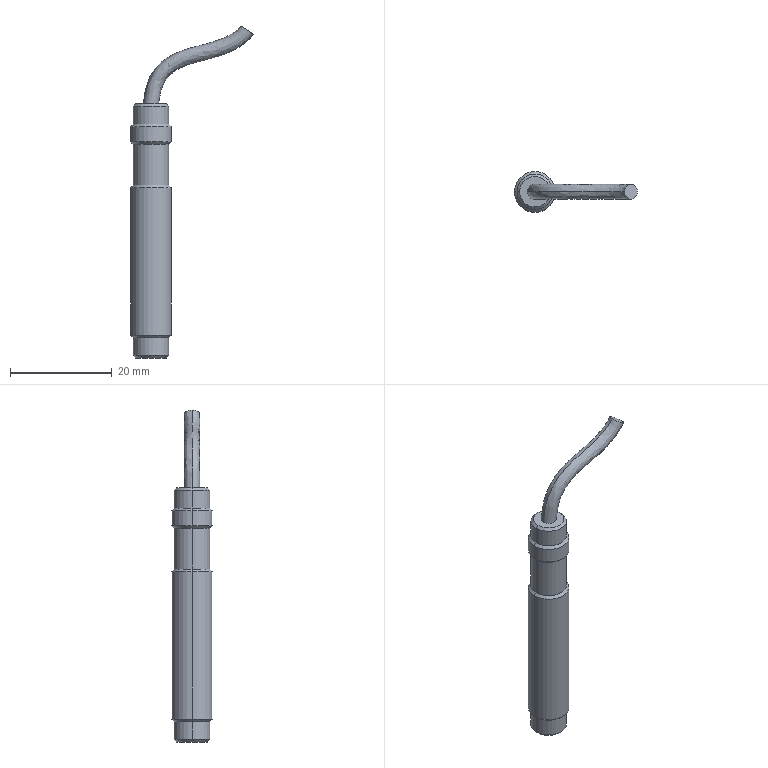Part | STEP file | 11-PSC0802-N.11 | 1 solid | 27 faces | box 24.159 x 8 x 65.269 mm | volume 2489 mm3 | cone 12 | cylinder 10 | plane 3 | spline 2 | commonest cylinder face diameters 7 x6 8 x4
STEP:
#1=CARTESIAN_POINT('',(3.5,0.,4.));
#2=VERTEX_POINT('',#1);
#3=CARTESIAN_POINT('',(-3.5,0.,4.));
#4=VERTEX_POINT('',#3);
#5=CARTESIAN_POINT('',(0.,0.,4.));
#6=DIRECTION('',(0.,0.,1.));
#7=DIRECTION('',(1.,0.,0.));
#8=AXIS2_PLACEMENT_3D('',#5,#6,#7);
#9=CIRCLE('',#8,3.5);
#10=EDGE_CURVE('',#2,#4,#9,.T.);
#11=ORIENTED_EDGE('',*,*,#10,.T.);
#12=CARTESIAN_POINT('',(-4.,0.,4.5));
#13=VERTEX_POINT('',#12);
#14=CARTESIAN_POINT('',(-4.,0.,4.5));
#15=DIRECTION('',(-0.7071,0.,0.7071));
#16=VECTOR('',#15,1000.);
#17=LINE('',#14,#16);
#18=EDGE_CURVE('',#4,#13,#17,.T.);
#19=ORIENTED_EDGE('',*,*,#18,.T.);
#20=CARTESIAN_POINT('',(4.,0.,4.5));
#21=VERTEX_POINT('',#20);
#22=CARTESIAN_POINT('',(0.,0.,4.5));
#23=DIRECTION('',(0.,0.,1.));
#24=DIRECTION('',(1.,0.,0.));
#25=AXIS2_PLACEMENT_3D('',#22,#23,#24);
#26=CIRCLE('',#25,4.);
#27=EDGE_CURVE('',#21,#13,#26,.T.);
#28=ORIENTED_EDGE('',*,*,#27,.F.);
#29=CARTESIAN_POINT('',(4.,0.,4.5));
#30=DIRECTION('',(0.7071,0.,0.7071));
#31=VECTOR('',#30,1000.);
#32=LINE('',#29,#31);
#33=EDGE_CURVE('',#2,#21,#32,.T.);
#34=ORIENTED_EDGE('',*,*,#33,.F.);
#35=EDGE_LOOP('',(#11,#19,#28,#34));
#36=FACE_OUTER_BOUND('',#35,.T.);
#37=CARTESIAN_POINT('',(0.,0.,4.5));
#38=DIRECTION('',(0.,0.,1.));
#39=DIRECTION('',(1.,0.,0.));
#40=AXIS2_PLACEMENT_3D('',#37,#38,#39);
#41=CONICAL_SURFACE('',#40,4.,0.7854);
#42=ADVANCED_FACE('',(#36),#41,.T.);
#43=CARTESIAN_POINT('',(3.5,0.,34.));
#44=VERTEX_POINT('',#43);
#45=CARTESIAN_POINT('',(-3.5,0.,34.));
#46=VERTEX_POINT('',#45);
#47=CARTESIAN_POINT('',(0.,0.,34.));
#48=DIRECTION('',(0.,0.,1.));
#49=DIRECTION('',(1.,0.,0.));
#50=AXIS2_PLACEMENT_3D('',#47,#48,#49);
#51=CIRCLE('',#50,3.5);
#52=EDGE_CURVE('',#44,#46,#51,.T.);
#53=ORIENTED_EDGE('',*,*,#52,.F.);
#54=CARTESIAN_POINT('',(4.,0.,33.5));
#55=VERTEX_POINT('',#54);
#56=CARTESIAN_POINT('',(3.5,0.,34.));
#57=DIRECTION('',(0.7071,0.,-0.7071));
#58=VECTOR('',#57,1000.);
#59=LINE('',#56,#58);
#60=EDGE_CURVE('',#44,#55,#59,.T.);
#61=ORIENTED_EDGE('',*,*,#60,.T.);
#62=CARTESIAN_POINT('',(-4.,0.,33.5));
#63=VERTEX_POINT('',#62);
#64=CARTESIAN_POINT('',(0.,0.,33.5));
#65=DIRECTION('',(0.,0.,-1.));
#66=DIRECTION('',(1.,0.,0.));
#67=AXIS2_PLACEMENT_3D('',#64,#65,#66);
#68=CIRCLE('',#67,4.);
#69=EDGE_CURVE('',#63,#55,#68,.T.);
#70=ORIENTED_EDGE('',*,*,#69,.F.);
#71=CARTESIAN_POINT('',(-3.5,0.,34.));
#72=DIRECTION('',(-0.7071,0.,-0.7071));
#73=VECTOR('',#72,1000.);
#74=LINE('',#71,#73);
#75=EDGE_CURVE('',#46,#63,#74,.T.);
#76=ORIENTED_EDGE('',*,*,#75,.F.);
#77=EDGE_LOOP('',(#53,#61,#70,#76));
#78=FACE_OUTER_BOUND('',#77,.T.);
#79=CARTESIAN_POINT('',(0.,0.,34.));
#80=DIRECTION('',(0.,0.,-1.));
#81=DIRECTION('',(-1.,0.,0.));
#82=AXIS2_PLACEMENT_3D('',#79,#80,#81);
#83=CONICAL_SURFACE('',#82,3.5,0.7854);
#84=ADVANCED_FACE('',(#78),#83,.T.);
#85=CARTESIAN_POINT('',(-3.,0.,0.));
#86=VERTEX_POINT('',#85);
#87=CARTESIAN_POINT('',(3.,0.,0.));
#88=VERTEX_POINT('',#87);
#89=CARTESIAN_POINT('',(0.,0.,0.));
#90=DIRECTION('',(0.,0.,-1.));
#91=DIRECTION('',(1.,0.,0.));
#92=AXIS2_PLACEMENT_3D('',#89,#90,#91);
#93=CIRCLE('',#92,3.);
#94=EDGE_CURVE('',#86,#88,#93,.T.);
#95=ORIENTED_EDGE('',*,*,#94,.F.);
#96=CARTESIAN_POINT('',(-3.5,0.,0.5));
#97=VERTEX_POINT('',#96);
#98=CARTESIAN_POINT('',(-3.5,0.,0.5));
#99=DIRECTION('',(-0.7071,0.,0.7071));
#100=VECTOR('',#99,1000.);
#101=LINE('',#98,#100);
#102=EDGE_CURVE('',#86,#97,#101,.T.);
#103=ORIENTED_EDGE('',*,*,#102,.T.);
#104=CARTESIAN_POINT('',(3.5,0.,0.5));
#105=VERTEX_POINT('',#104);
#106=CARTESIAN_POINT('',(0.,0.,0.5));
#107=DIRECTION('',(0.,0.,1.));
#108=DIRECTION('',(1.,0.,0.));
#109=AXIS2_PLACEMENT_3D('',#106,#107,#108);
#110=CIRCLE('',#109,3.5);
#111=EDGE_CURVE('',#105,#97,#110,.T.);
#112=ORIENTED_EDGE('',*,*,#111,.F.);
#113=CARTESIAN_POINT('',(3.5,0.,0.5));
#114=DIRECTION('',(0.7071,0.,0.7071));
#115=VECTOR('',#114,1000.);
#116=LINE('',#113,#115);
#117=EDGE_CURVE('',#88,#105,#116,.T.);
#118=ORIENTED_EDGE('',*,*,#117,.F.);
#119=EDGE_LOOP('',(#95,#103,#112,#118));
#120=FACE_OUTER_BOUND('',#119,.T.);
#121=CARTESIAN_POINT('',(0.,0.,0.5));
#122=DIRECTION('',(0.,0.,1.));
#123=DIRECTION('',(1.,0.,0.));
#124=AXIS2_PLACEMENT_3D('',#121,#122,#123);
#125=CONICAL_SURFACE('',#124,3.5,0.7854);
#126=ADVANCED_FACE('',(#120),#125,.T.);
#127=CARTESIAN_POINT('',(3.5,0.,42.));
#128=VERTEX_POINT('',#127);
#129=CARTESIAN_POINT('',(-3.5,0.,42.));
#130=VERTEX_POINT('',#129);
#131=CARTESIAN_POINT('',(0.,0.,42.));
#132=DIRECTION('',(0.,0.,1.));
#133=DIRECTION('',(1.,0.,0.));
#134=AXIS2_PLACEMENT_3D('',#131,#132,#133);
#135=CIRCLE('',#134,3.5);
#136=EDGE_CURVE('',#128,#130,#135,.T.);
#137=ORIENTED_EDGE('',*,*,#136,.T.);
#138=CARTESIAN_POINT('',(-4.,0.,42.5));
#139=VERTEX_POINT('',#138);
#140=CARTESIAN_POINT('',(-4.,0.,42.5));
#141=DIRECTION('',(-0.7071,0.,0.7071));
#142=VECTOR('',#141,1000.);
#143=LINE('',#140,#142);
#144=EDGE_CURVE('',#130,#139,#143,.T.);
#145=ORIENTED_EDGE('',*,*,#144,.T.);
#146=CARTESIAN_POINT('',(4.,0.,42.5));
#147=VERTEX_POINT('',#146);
#148=CARTESIAN_POINT('',(0.,0.,42.5));
#149=DIRECTION('',(0.,0.,1.));
#150=DIRECTION('',(1.,0.,0.));
#151=AXIS2_PLACEMENT_3D('',#148,#149,#150);
#152=CIRCLE('',#151,4.);
#153=EDGE_CURVE('',#147,#139,#152,.T.);
#154=ORIENTED_EDGE('',*,*,#153,.F.);
#155=CARTESIAN_POINT('',(4.,0.,42.5));
#156=DIRECTION('',(0.7071,0.,0.7071));
#157=VECTOR('',#156,1000.);
#158=LINE('',#155,#157);
#159=EDGE_CURVE('',#128,#147,#158,.T.);
#160=ORIENTED_EDGE('',*,*,#159,.F.);
#161=EDGE_LOOP('',(#137,#145,#154,#160));
#162=FACE_OUTER_BOUND('',#161,.T.);
#163=CARTESIAN_POINT('',(0.,0.,42.5));
#164=DIRECTION('',(0.,0.,1.));
#165=DIRECTION('',(1.,0.,0.));
#166=AXIS2_PLACEMENT_3D('',#163,#164,#165);
#167=CONICAL_SURFACE('',#166,4.,0.7854);
#168=ADVANCED_FACE('',(#162),#167,.T.);
#169=CARTESIAN_POINT('',(3.5,0.,46.));
#170=VERTEX_POINT('',#169);
#171=CARTESIAN_POINT('',(-3.5,0.,46.));
#172=VERTEX_POINT('',#171);
#173=CARTESIAN_POINT('',(0.,0.,46.));
#174=DIRECTION('',(0.,0.,1.));
#175=DIRECTION('',(1.,0.,0.));
#176=AXIS2_PLACEMENT_3D('',#173,#174,#175);
#177=CIRCLE('',#176,3.5);
#178=EDGE_CURVE('',#170,#172,#177,.T.);
#179=ORIENTED_EDGE('',*,*,#178,.F.);
#180=CARTESIAN_POINT('',(4.,0.,45.5));
#181=VERTEX_POINT('',#180);
#182=CARTESIAN_POINT('',(3.5,0.,46.));
#183=DIRECTION('',(0.7071,0.,-0.7071));
#184=VECTOR('',#183,1000.);
#185=LINE('',#182,#184);
#186=EDGE_CURVE('',#170,#181,#185,.T.);
#187=ORIENTED_EDGE('',*,*,#186,.T.);
#188=CARTESIAN_POINT('',(-4.,0.,45.5));
#189=VERTEX_POINT('',#188);
#190=CARTESIAN_POINT('',(0.,0.,45.5));
#191=DIRECTION('',(0.,0.,-1.));
#192=DIRECTION('',(1.,0.,0.));
#193=AXIS2_PLACEMENT_3D('',#190,#191,#192);
#194=CIRCLE('',#193,4.);
#195=EDGE_CURVE('',#189,#181,#194,.T.);
#196=ORIENTED_EDGE('',*,*,#195,.F.);
#197=CARTESIAN_POINT('',(-3.5,0.,46.));
#198=DIRECTION('',(-0.7071,0.,-0.7071));
#199=VECTOR('',#198,1000.);
#200=LINE('',#197,#199);
#201=EDGE_CURVE('',#172,#189,#200,.T.);
#202=ORIENTED_EDGE('',*,*,#201,.F.);
#203=EDGE_LOOP('',(#179,#187,#196,#202));
#204=FACE_OUTER_BOUND('',#203,.T.);
#205=CARTESIAN_POINT('',(0.,0.,46.));
#206=DIRECTION('',(0.,0.,-1.));
#207=DIRECTION('',(-1.,0.,0.));
#208=AXIS2_PLACEMENT_3D('',#205,#206,#207);
#209=CONICAL_SURFACE('',#208,3.5,0.7854);
#210=ADVANCED_FACE('',(#204),#209,.T.);
#211=CARTESIAN_POINT('',(3.,0.,50.));
#212=VERTEX_POINT('',#211);
#213=CARTESIAN_POINT('',(-3.,0.,50.));
#214=VERTEX_POINT('',#213);
#215=CARTESIAN_POINT('',(0.,0.,50.));
#216=DIRECTION('',(0.,0.,1.));
#217=DIRECTION('',(1.,0.,0.));
#218=AXIS2_PLACEMENT_3D('',#215,#216,#217);
#219=CIRCLE('',#218,3.);
#220=EDGE_CURVE('',#212,#214,#219,.T.);
#221=ORIENTED_EDGE('',*,*,#220,.F.);
#222=CARTESIAN_POINT('',(3.5,0.,49.5));
#223=VERTEX_POINT('',#222);
#224=CARTESIAN_POINT('',(3.,0.,50.));
#225=DIRECTION('',(0.7071,0.,-0.7071));
#226=VECTOR('',#225,1000.);
#227=LINE('',#224,#226);
#228=EDGE_CURVE('',#212,#223,#227,.T.);
#229=ORIENTED_EDGE('',*,*,#228,.T.);
#230=CARTESIAN_POINT('',(-3.5,0.,49.5));
#231=VERTEX_POINT('',#230);
#232=CARTESIAN_POINT('',(0.,0.,49.5));
#233=DIRECTION('',(0.,0.,-1.));
#234=DIRECTION('',(1.,0.,0.));
#235=AXIS2_PLACEMENT_3D('',#232,#233,#234);
#236=CIRCLE('',#235,3.5);
#237=EDGE_CURVE('',#231,#223,#236,.T.);
#238=ORIENTED_EDGE('',*,*,#237,.F.);
#239=CARTESIAN_POINT('',(-3.,0.,50.));
#240=DIRECTION('',(-0.7071,0.,-0.7071));
#241=VECTOR('',#240,1000.);
#242=LINE('',#239,#241);
#243=EDGE_CURVE('',#214,#231,#242,.T.);
#244=ORIENTED_EDGE('',*,*,#243,.F.);
#245=EDGE_LOOP('',(#221,#229,#238,#244));
#246=FACE_OUTER_BOUND('',#245,.T.);
#247=CARTESIAN_POINT('',(0.,0.,50.));
#248=DIRECTION('',(0.,0.,-1.));
#249=DIRECTION('',(-1.,0.,0.));
#250=AXIS2_PLACEMENT_3D('',#247,#248,#249);
#251=CONICAL_SURFACE('',#250,3.,0.7854);
#252=ADVANCED_FACE('',(#246),#251,.T.);
#253=CARTESIAN_POINT('',(1.5,0.,50.));
#254=VERTEX_POINT('',#253);
#255=CARTESIAN_POINT('',(-1.5,0.,50.));
#256=VERTEX_POINT('',#255);
#257=CARTESIAN_POINT('',(0.,0.,50.));
#258=DIRECTION('',(0.,0.,1.));
#259=DIRECTION('',(0.,-1.,0.));
#260=AXIS2_PLACEMENT_3D('',#257,#258,#259);
#261=CIRCLE('',#260,1.5);
#262=EDGE_CURVE('',#254,#256,#261,.T.);
#263=ORIENTED_EDGE('',*,*,#262,.T.);
#264=CARTESIAN_POINT('',(17.659,0.,65.269));
#265=VERTEX_POINT('',#264);
#266=CARTESIAN_POINT('',(-1.5,0.,50.));
#267=CARTESIAN_POINT('',(-1.453,0.,50.688));
#268=CARTESIAN_POINT('',(-1.301,0.,51.976));
#269=CARTESIAN_POINT('',(-0.8799,0.,53.698));
#270=CARTESIAN_POINT('',(-0.2755,0.,55.215));
#271=CARTESIAN_POINT('',(0.5036,0.,56.534));
#272=CARTESIAN_POINT('',(1.902,0.,58.214));
#273=CARTESIAN_POINT('',(4.18,0.,59.765));
#274=CARTESIAN_POINT('',(7.284,0.,60.869));
#275=CARTESIAN_POINT('',(10.404,0.,61.626));
#276=CARTESIAN_POINT('',(13.333,0.,62.4));
#277=CARTESIAN_POINT('',(15.815,0.,63.5));
#278=CARTESIAN_POINT('',(17.122,0.,64.555));
#279=CARTESIAN_POINT('',(17.659,0.,65.269));
#280=B_SPLINE_CURVE_WITH_KNOTS('',3,(#266,#267,#268,#269,#270,#271,#272,#273,#274,#275,#276,#277,#278,#279),.UNSPECIFIED.,.F.,.F.,(4,1,1,1,1,1,1,1,1,1,1,4),(0.,0.05,0.1,0.15,0.2,0.25,0.375,0.5,0.625,0.75,0.875,1.),.UNSPECIFIED.);
#281=EDGE_CURVE('',#256,#265,#280,.T.);
#282=ORIENTED_EDGE('',*,*,#281,.T.);
#283=CARTESIAN_POINT('',(20.159,0.,63.611));
#284=VERTEX_POINT('',#283);
#285=CARTESIAN_POINT('',(18.909,0.,64.44));
#286=DIRECTION('',(-0.5528,0.,-0.8333));
#287=DIRECTION('',(-0.8333,0.,0.5528));
#288=AXIS2_PLACEMENT_3D('',#285,#286,#287);
#289=CIRCLE('',#288,1.5);
#290=EDGE_CURVE('',#265,#284,#289,.T.);
#291=ORIENTED_EDGE('',*,*,#290,.T.);
#292=CARTESIAN_POINT('',(1.5,0.,50.));
#293=CARTESIAN_POINT('',(1.544,0.,50.58));
#294=CARTESIAN_POINT('',(1.69,0.,51.651));
#295=CARTESIAN_POINT('',(2.043,0.,52.978));
#296=CARTESIAN_POINT('',(2.509,0.,54.065));
#297=CARTESIAN_POINT('',(3.069,0.,54.952));
#298=CARTESIAN_POINT('',(4.037,0.,56.048));
#299=CARTESIAN_POINT('',(5.651,0.,57.113));
#300=CARTESIAN_POINT('',(8.273,0.,58.035));
#301=CARTESIAN_POINT('',(11.291,0.,58.759));
#302=CARTESIAN_POINT('',(14.458,0.,59.614));
#303=CARTESIAN_POINT('',(17.578,0.,60.989));
#304=CARTESIAN_POINT('',(19.376,0.,62.612));
#305=CARTESIAN_POINT('',(20.159,0.,63.611));
#306=B_SPLINE_CURVE_WITH_KNOTS('',3,(#292,#293,#294,#295,#296,#297,#298,#299,#300,#301,#302,#303,#304,#305),.UNSPECIFIED.,.F.,.F.,(4,1,1,1,1,1,1,1,1,1,1,4),(0.,0.05,0.1,0.15,0.2,0.25,0.375,0.5,0.625,0.75,0.875,1.),.UNSPECIFIED.);
#307=EDGE_CURVE('',#254,#284,#306,.T.);
#308=ORIENTED_EDGE('',*,*,#307,.F.);
#309=EDGE_LOOP('',(#263,#282,#291,#308));
#310=FACE_OUTER_BOUND('',#309,.T.);
#311=CARTESIAN_POINT('',(1.5,0.,50.));
#312=CARTESIAN_POINT('',(1.544,0.,50.58));
#313=CARTESIAN_POINT('',(1.69,0.,51.651));
#314=CARTESIAN_POINT('',(2.043,0.,52.978));
#315=CARTESIAN_POINT('',(2.509,0.,54.065));
#316=CARTESIAN_POINT('',(3.069,0.,54.952));
#317=CARTESIAN_POINT('',(4.037,0.,56.048));
#318=CARTESIAN_POINT('',(5.651,0.,57.113));
#319=CARTESIAN_POINT('',(8.273,0.,58.035));
#320=CARTESIAN_POINT('',(11.291,0.,58.759));
#321=CARTESIAN_POINT('',(14.458,0.,59.614));
#322=CARTESIAN_POINT('',(17.578,0.,60.989));
#323=CARTESIAN_POINT('',(19.376,0.,62.612));
#324=CARTESIAN_POINT('',(20.159,0.,63.611));
#325=CARTESIAN_POINT('',(1.5,3.,50.));
#326=CARTESIAN_POINT('',(1.544,3.,50.58));
#327=CARTESIAN_POINT('',(1.69,3.,51.651));
#328=CARTESIAN_POINT('',(2.043,3.,52.978));
#329=CARTESIAN_POINT('',(2.509,3.,54.065));
#330=CARTESIAN_POINT('',(3.069,3.,54.952));
#331=CARTESIAN_POINT('',(4.037,3.,56.048));
#332=CARTESIAN_POINT('',(5.651,3.,57.113));
#333=CARTESIAN_POINT('',(8.273,3.,58.035));
#334=CARTESIAN_POINT('',(11.291,3.,58.759));
#335=CARTESIAN_POINT('',(14.458,3.,59.614));
#336=CARTESIAN_POINT('',(17.578,3.,60.989));
#337=CARTESIAN_POINT('',(19.376,3.,62.612));
#338=CARTESIAN_POINT('',(20.159,3.,63.611));
#339=CARTESIAN_POINT('',(-1.5,3.,50.));
#340=CARTESIAN_POINT('',(-1.453,3.,50.688));
#341=CARTESIAN_POINT('',(-1.301,3.,51.976));
#342=CARTESIAN_POINT('',(-0.8799,3.,53.698));
#343=CARTESIAN_POINT('',(-0.2755,3.,55.215));
#344=CARTESIAN_POINT('',(0.5036,3.,56.534));
#345=CARTESIAN_POINT('',(1.902,3.,58.214));
#346=CARTESIAN_POINT('',(4.18,3.,59.765));
#347=CARTESIAN_POINT('',(7.284,3.,60.869));
#348=CARTESIAN_POINT('',(10.404,3.,61.626));
#349=CARTESIAN_POINT('',(13.333,3.,62.4));
#350=CARTESIAN_POINT('',(15.815,3.,63.5));
#351=CARTESIAN_POINT('',(17.122,3.,64.555));
#352=CARTESIAN_POINT('',(17.659,3.,65.269));
#353=CARTESIAN_POINT('',(-1.5,0.,50.));
#354=CARTESIAN_POINT('',(-1.453,0.,50.688));
#355=CARTESIAN_POINT('',(-1.301,0.,51.976));
#356=CARTESIAN_POINT('',(-0.8799,0.,53.698));
#357=CARTESIAN_POINT('',(-0.2755,0.,55.215));
#358=CARTESIAN_POINT('',(0.5036,0.,56.534));
#359=CARTESIAN_POINT('',(1.902,0.,58.214));
#360=CARTESIAN_POINT('',(4.18,0.,59.765));
#361=CARTESIAN_POINT('',(7.284,0.,60.869));
#362=CARTESIAN_POINT('',(10.404,0.,61.626));
#363=CARTESIAN_POINT('',(13.333,0.,62.4));
#364=CARTESIAN_POINT('',(15.815,0.,63.5));
#365=CARTESIAN_POINT('',(17.122,0.,64.555));
#366=CARTESIAN_POINT('',(17.659,0.,65.269));
#367=CARTESIAN_POINT('',(-1.5,-3.,50.));
#368=CARTESIAN_POINT('',(-1.453,-3.,50.688));
#369=CARTESIAN_POINT('',(-1.301,-3.,51.976));
#370=CARTESIAN_POINT('',(-0.8799,-3.,53.698));
#371=CARTESIAN_POINT('',(-0.2755,-3.,55.215));
#372=CARTESIAN_POINT('',(0.5036,-3.,56.534));
#373=CARTESIAN_POINT('',(1.902,-3.,58.214));
#374=CARTESIAN_POINT('',(4.18,-3.,59.765));
#375=CARTESIAN_POINT('',(7.284,-3.,60.869));
#376=CARTESIAN_POINT('',(10.404,-3.,61.626));
#377=CARTESIAN_POINT('',(13.333,-3.,62.4));
#378=CARTESIAN_POINT('',(15.815,-3.,63.5));
#379=CARTESIAN_POINT('',(17.122,-3.,64.555));
#380=CARTESIAN_POINT('',(17.659,-3.,65.269));
#381=CARTESIAN_POINT('',(1.5,-3.,50.));
#382=CARTESIAN_POINT('',(1.544,-3.,50.58));
#383=CARTESIAN_POINT('',(1.69,-3.,51.651));
#384=CARTESIAN_POINT('',(2.043,-3.,52.978));
#385=CARTESIAN_POINT('',(2.509,-3.,54.065));
#386=CARTESIAN_POINT('',(3.069,-3.,54.952));
#387=CARTESIAN_POINT('',(4.037,-3.,56.048));
#388=CARTESIAN_POINT('',(5.651,-3.,57.113));
#389=CARTESIAN_POINT('',(8.273,-3.,58.035));
#390=CARTESIAN_POINT('',(11.291,-3.,58.759));
#391=CARTESIAN_POINT('',(14.458,-3.,59.614));
#392=CARTESIAN_POINT('',(17.578,-3.,60.989));
#393=CARTESIAN_POINT('',(19.376,-3.,62.612));
#394=CARTESIAN_POINT('',(20.159,-3.,63.611));
#395=CARTESIAN_POINT('',(1.5,0.,50.));
#396=CARTESIAN_POINT('',(1.544,0.,50.58));
#397=CARTESIAN_POINT('',(1.69,0.,51.651));
#398=CARTESIAN_POINT('',(2.043,0.,52.978));
#399=CARTESIAN_POINT('',(2.509,0.,54.065));
#400=CARTESIAN_POINT('',(3.069,0.,54.952));
#401=CARTESIAN_POINT('',(4.037,0.,56.048));
#402=CARTESIAN_POINT('',(5.651,0.,57.113));
#403=CARTESIAN_POINT('',(8.273,0.,58.035));
#404=CARTESIAN_POINT('',(11.291,0.,58.759));
#405=CARTESIAN_POINT('',(14.458,0.,59.614));
#406=CARTESIAN_POINT('',(17.578,0.,60.989));
#407=CARTESIAN_POINT('',(19.376,0.,62.612));
#408=CARTESIAN_POINT('',(20.159,0.,63.611));
#409=(BOUNDED_SURFACE()B_SPLINE_SURFACE(3,3,((#311,#312,#313,#314,#315,#316,#317,#318,#319,#320,#321,#322,#323,#324),(#325,#326,#327,#328,#329,#330,#331,#332,#333,#334,#335,#336,#337,#338),(#339,#340,#341,#342,#343,#344,#345,#346,#347,#348,#349,#350,#351,#352),(#353,#354,#355,#356,#357,#358,#359,#360,#361,#362,#363,#364,#365,#366),(#367,#368,#369,#370,#371,#372,#373,#374,#375,#376,#377,#378,#379,#380),(#381,#382,#383,#384,#385,#386,#387,#388,#389,#390,#391,#392,#393,#394),(#395,#396,#397,#398,#399,#400,#401,#402,#403,#404,#405,#406,#407,#408)),.UNSPECIFIED.,.T.,.F.,.F.)B_SPLINE_SURFACE_WITH_KNOTS((4,3,4),(4,1,1,1,1,1,1,1,1,1,1,4),(0.,0.5,1.),(0.,0.05,0.1,0.15,0.2,0.25,0.375,0.5,0.625,0.75,0.875,1.),.UNSPECIFIED.)GEOMETRIC_REPRESENTATION_ITEM()RATIONAL_B_SPLINE_SURFACE(((1.,1.,1.,1.,1.,1.,1.,1.,1.,1.,1.,1.,1.,1.),(0.3333,0.3333,0.3333,0.3333,0.3333,0.3333,0.3333,0.3333,0.3333,0.3333,0.3333,0.3333,0.3333,0.3333),(0.3333,0.3333,0.3333,0.3333,0.3333,0.3333,0.3333,0.3333,0.3333,0.3333,0.3333,0.3333,0.3333,0.3333),(1.,1.,1.,1.,1.,1.,1.,1.,1.,1.,1.,1.,1.,1.),(0.3333,0.3333,0.3333,0.3333,0.3333,0.3333,0.3333,0.3333,0.3333,0.3333,0.3333,0.3333,0.3333,0.3333),(0.3333,0.3333,0.3333,0.3333,0.3333,0.3333,0.3333,0.3333,0.3333,0.3333,0.3333,0.3333,0.3333,0.3333),(1.,1.,1.,1.,1.,1.,1.,1.,1.,1.,1.,1.,1.,1.)))REPRESENTATION_ITEM('')SURFACE());
#410=ADVANCED_FACE('',(#310),#409,.T.);
#411=ORIENTED_EDGE('',*,*,#237,.T.);
#412=CARTESIAN_POINT('',(3.5,0.,50.));
#413=DIRECTION('',(0.,0.,-1.));
#414=VECTOR('',#413,1000.);
#415=LINE('',#412,#414);
#416=EDGE_CURVE('',#223,#170,#415,.T.);
#417=ORIENTED_EDGE('',*,*,#416,.T.);
#418=ORIENTED_EDGE('',*,*,#178,.T.);
#419=CARTESIAN_POINT('',(-3.5,0.,50.));
#420=DIRECTION('',(0.,0.,-1.));
#421=VECTOR('',#420,1000.);
#422=LINE('',#419,#421);
#423=EDGE_CURVE('',#231,#172,#422,.T.);
#424=ORIENTED_EDGE('',*,*,#423,.F.);
#425=EDGE_LOOP('',(#411,#417,#418,#424));
#426=FACE_OUTER_BOUND('',#425,.T.);
#427=CARTESIAN_POINT('',(0.,0.,50.));
#428=DIRECTION('',(0.,0.,-1.));
#429=DIRECTION('',(-1.,0.,0.));
#430=AXIS2_PLACEMENT_3D('',#427,#428,#429);
#431=CYLINDRICAL_SURFACE('',#430,3.5);
#432=ADVANCED_FACE('',(#426),#431,.T.);
#433=ORIENTED_EDGE('',*,*,#195,.T.);
#434=CARTESIAN_POINT('',(4.,0.,46.));
#435=DIRECTION('',(0.,0.,-1.));
#436=VECTOR('',#435,1000.);
#437=LINE('',#434,#436);
#438=EDGE_CURVE('',#181,#147,#437,.T.);
#439=ORIENTED_EDGE('',*,*,#438,.T.);
#440=ORIENTED_EDGE('',*,*,#153,.T.);
#441=CARTESIAN_POINT('',(-4.,0.,46.));
#442=DIRECTION('',(0.,0.,-1.));
#443=VECTOR('',#442,1000.);
#444=LINE('',#441,#443);
#445=EDGE_CURVE('',#189,#139,#444,.T.);
#446=ORIENTED_EDGE('',*,*,#445,.F.);
#447=EDGE_LOOP('',(#433,#439,#440,#446));
#448=FACE_OUTER_BOUND('',#447,.T.);
#449=CARTESIAN_POINT('',(0.,0.,46.));
#450=DIRECTION('',(0.,0.,-1.));
#451=DIRECTION('',(-1.,0.,0.));
#452=AXIS2_PLACEMENT_3D('',#449,#450,#451);
#453=CYLINDRICAL_SURFACE('',#452,4.);
#454=ADVANCED_FACE('',(#448),#453,.T.);
#455=ORIENTED_EDGE('',*,*,#136,.F.);
#456=CARTESIAN_POINT('',(3.5,0.,42.));
#457=DIRECTION('',(0.,0.,-1.));
#458=VECTOR('',#457,1000.);
#459=LINE('',#456,#458);
#460=EDGE_CURVE('',#128,#44,#459,.T.);
#461=ORIENTED_EDGE('',*,*,#460,.T.);
#462=ORIENTED_EDGE('',*,*,#52,.T.);
#463=CARTESIAN_POINT('',(-3.5,0.,42.));
#464=DIRECTION('',(0.,0.,-1.));
#465=VECTOR('',#464,1000.);
#466=LINE('',#463,#465);
#467=EDGE_CURVE('',#130,#46,#466,.T.);
#468=ORIENTED_EDGE('',*,*,#467,.F.);
#469=EDGE_LOOP('',(#455,#461,#462,#468));
#470=FACE_OUTER_BOUND('',#469,.T.);
#471=CARTESIAN_POINT('',(0.,0.,42.));
#472=DIRECTION('',(0.,0.,-1.));
#473=DIRECTION('',(-1.,0.,0.));
#474=AXIS2_PLACEMENT_3D('',#471,#472,#473);
#475=CYLINDRICAL_SURFACE('',#474,3.5);
#476=ADVANCED_FACE('',(#470),#475,.T.);
#477=ORIENTED_EDGE('',*,*,#69,.T.);
#478=CARTESIAN_POINT('',(4.,0.,34.));
#479=DIRECTION('',(0.,0.,-1.));
#480=VECTOR('',#479,1000.);
#481=LINE('',#478,#480);
#482=EDGE_CURVE('',#55,#21,#481,.T.);
#483=ORIENTED_EDGE('',*,*,#482,.T.);
#484=ORIENTED_EDGE('',*,*,#27,.T.);
#485=CARTESIAN_POINT('',(-4.,0.,34.));
#486=DIRECTION('',(0.,0.,-1.));
#487=VECTOR('',#486,1000.);
#488=LINE('',#485,#487);
#489=EDGE_CURVE('',#63,#13,#488,.T.);
#490=ORIENTED_EDGE('',*,*,#489,.F.);
#491=EDGE_LOOP('',(#477,#483,#484,#490));
#492=FACE_OUTER_BOUND('',#491,.T.);
#493=CARTESIAN_POINT('',(0.,0.,34.));
#494=DIRECTION('',(0.,0.,-1.));
#495=DIRECTION('',(-1.,0.,0.));
#496=AXIS2_PLACEMENT_3D('',#493,#494,#495);
#497=CYLINDRICAL_SURFACE('',#496,4.);
#498=ADVANCED_FACE('',(#492),#497,.T.);
#499=ORIENTED_EDGE('',*,*,#10,.F.);
#500=CARTESIAN_POINT('',(3.5,0.,4.));
#501=DIRECTION('',(0.,0.,-1.));
#502=VECTOR('',#501,1000.);
#503=LINE('',#500,#502);
#504=EDGE_CURVE('',#2,#105,#503,.T.);
#505=ORIENTED_EDGE('',*,*,#504,.T.);
#506=ORIENTED_EDGE('',*,*,#111,.T.);
#507=CARTESIAN_POINT('',(-3.5,0.,4.));
#508=DIRECTION('',(0.,0.,-1.));
#509=VECTOR('',#508,1000.);
#510=LINE('',#507,#509);
#511=EDGE_CURVE('',#4,#97,#510,.T.);
#512=ORIENTED_EDGE('',*,*,#511,.F.);
#513=EDGE_LOOP('',(#499,#505,#506,#512));
#514=FACE_OUTER_BOUND('',#513,.T.);
#515=CARTESIAN_POINT('',(0.,0.,4.));
#516=DIRECTION('',(0.,0.,-1.));
#517=DIRECTION('',(-1.,0.,0.));
#518=AXIS2_PLACEMENT_3D('',#515,#516,#517);
#519=CYLINDRICAL_SURFACE('',#518,3.5);
#520=ADVANCED_FACE('',(#514),#519,.T.);
#521=ORIENTED_EDGE('',*,*,#504,.F.);
#522=CARTESIAN_POINT('',(0.,0.,4.));
#523=DIRECTION('',(0.,0.,1.));
#524=DIRECTION('',(1.,0.,0.));
#525=AXIS2_PLACEMENT_3D('',#522,#523,#524);
#526=CIRCLE('',#525,3.5);
#527=EDGE_CURVE('',#4,#2,#526,.T.);
#528=ORIENTED_EDGE('',*,*,#527,.F.);
#529=ORIENTED_EDGE('',*,*,#511,.T.);
#530=CARTESIAN_POINT('',(0.,0.,0.5));
#531=DIRECTION('',(0.,0.,1.));
#532=DIRECTION('',(1.,0.,0.));
#533=AXIS2_PLACEMENT_3D('',#530,#531,#532);
#534=CIRCLE('',#533,3.5);
#535=EDGE_CURVE('',#97,#105,#534,.T.);
#536=ORIENTED_EDGE('',*,*,#535,.T.);
#537=EDGE_LOOP('',(#521,#528,#529,#536));
#538=FACE_OUTER_BOUND('',#537,.T.);
#539=CARTESIAN_POINT('',(0.,0.,4.));
#540=DIRECTION('',(0.,0.,-1.));
#541=DIRECTION('',(-1.,0.,0.));
#542=AXIS2_PLACEMENT_3D('',#539,#540,#541);
#543=CYLINDRICAL_SURFACE('',#542,3.5);
#544=ADVANCED_FACE('',(#538),#543,.T.);
#545=CARTESIAN_POINT('',(0.,0.,0.));
#546=DIRECTION('',(0.,0.,-1.));
#547=DIRECTION('',(1.,0.,0.));
#548=AXIS2_PLACEMENT_3D('',#545,#546,#547);
#549=CIRCLE('',#548,3.);
#550=EDGE_CURVE('',#88,#86,#549,.T.);
#551=ORIENTED_EDGE('',*,*,#550,.T.);
#552=ORIENTED_EDGE('',*,*,#94,.T.);
#553=EDGE_LOOP('',(#551,#552));
#554=FACE_OUTER_BOUND('',#553,.T.);
#555=CARTESIAN_POINT('',(0.,0.,0.));
#556=DIRECTION('',(0.,0.,1.));
#557=DIRECTION('',(1.,0.,0.));
#558=AXIS2_PLACEMENT_3D('',#555,#556,#557);
#559=PLANE('',#558);
#560=ADVANCED_FACE('',(#554),#559,.F.);
#561=ORIENTED_EDGE('',*,*,#482,.F.);
#562=CARTESIAN_POINT('',(0.,0.,33.5));
#563=DIRECTION('',(0.,0.,-1.));
#564=DIRECTION('',(1.,0.,0.));
#565=AXIS2_PLACEMENT_3D('',#562,#563,#564);
#566=CIRCLE('',#565,4.);
#567=EDGE_CURVE('',#55,#63,#566,.T.);
#568=ORIENTED_EDGE('',*,*,#567,.T.);
#569=ORIENTED_EDGE('',*,*,#489,.T.);
#570=CARTESIAN_POINT('',(0.,0.,4.5));
#571=DIRECTION('',(0.,0.,1.));
#572=DIRECTION('',(1.,0.,0.));
#573=AXIS2_PLACEMENT_3D('',#570,#571,#572);
#574=CIRCLE('',#573,4.);
#575=EDGE_CURVE('',#13,#21,#574,.T.);
#576=ORIENTED_EDGE('',*,*,#575,.T.);
#577=EDGE_LOOP('',(#561,#568,#569,#576));
#578=FACE_OUTER_BOUND('',#577,.T.);
#579=CARTESIAN_POINT('',(0.,0.,34.));
#580=DIRECTION('',(0.,0.,-1.));
#581=DIRECTION('',(-1.,0.,0.));
#582=AXIS2_PLACEMENT_3D('',#579,#580,#581);
#583=CYLINDRICAL_SURFACE('',#582,4.);
#584=ADVANCED_FACE('',(#578),#583,.T.);
#585=ORIENTED_EDGE('',*,*,#460,.F.);
#586=CARTESIAN_POINT('',(0.,0.,42.));
#587=DIRECTION('',(0.,0.,1.));
#588=DIRECTION('',(1.,0.,0.));
#589=AXIS2_PLACEMENT_3D('',#586,#587,#588);
#590=CIRCLE('',#589,3.5);
#591=EDGE_CURVE('',#130,#128,#590,.T.);
#592=ORIENTED_EDGE('',*,*,#591,.F.);
#593=ORIENTED_EDGE('',*,*,#467,.T.);
#594=CARTESIAN_POINT('',(0.,0.,34.));
#595=DIRECTION('',(0.,0.,1.));
#596=DIRECTION('',(1.,0.,0.));
#597=AXIS2_PLACEMENT_3D('',#594,#595,#596);
#598=CIRCLE('',#597,3.5);
#599=EDGE_CURVE('',#46,#44,#598,.T.);
#600=ORIENTED_EDGE('',*,*,#599,.T.);
#601=EDGE_LOOP('',(#585,#592,#593,#600));
#602=FACE_OUTER_BOUND('',#601,.T.);
#603=CARTESIAN_POINT('',(0.,0.,42.));
#604=DIRECTION('',(0.,0.,-1.));
#605=DIRECTION('',(-1.,0.,0.));
#606=AXIS2_PLACEMENT_3D('',#603,#604,#605);
#607=CYLINDRICAL_SURFACE('',#606,3.5);
#608=ADVANCED_FACE('',(#602),#607,.T.);
#609=ORIENTED_EDGE('',*,*,#438,.F.);
#610=CARTESIAN_POINT('',(0.,0.,45.5));
#611=DIRECTION('',(0.,0.,-1.));
#612=DIRECTION('',(1.,0.,0.));
#613=AXIS2_PLACEMENT_3D('',#610,#611,#612);
#614=CIRCLE('',#613,4.);
#615=EDGE_CURVE('',#181,#189,#614,.T.);
#616=ORIENTED_EDGE('',*,*,#615,.T.);
#617=ORIENTED_EDGE('',*,*,#445,.T.);
#618=CARTESIAN_POINT('',(0.,0.,42.5));
#619=DIRECTION('',(0.,0.,1.));
#620=DIRECTION('',(1.,0.,0.));
#621=AXIS2_PLACEMENT_3D('',#618,#619,#620);
#622=CIRCLE('',#621,4.);
#623=EDGE_CURVE('',#139,#147,#622,.T.);
#624=ORIENTED_EDGE('',*,*,#623,.T.);
#625=EDGE_LOOP('',(#609,#616,#617,#624));
#626=FACE_OUTER_BOUND('',#625,.T.);
#627=CARTESIAN_POINT('',(0.,0.,46.));
#628=DIRECTION('',(0.,0.,-1.));
#629=DIRECTION('',(-1.,0.,0.));
#630=AXIS2_PLACEMENT_3D('',#627,#628,#629);
#631=CYLINDRICAL_SURFACE('',#630,4.);
#632=ADVANCED_FACE('',(#626),#631,.T.);
#633=ORIENTED_EDGE('',*,*,#416,.F.);
#634=CARTESIAN_POINT('',(0.,0.,49.5));
#635=DIRECTION('',(0.,0.,-1.));
#636=DIRECTION('',(1.,0.,0.));
#637=AXIS2_PLACEMENT_3D('',#634,#635,#636);
#638=CIRCLE('',#637,3.5);
#639=EDGE_CURVE('',#223,#231,#638,.T.);
#640=ORIENTED_EDGE('',*,*,#639,.T.);
#641=ORIENTED_EDGE('',*,*,#423,.T.);
#642=CARTESIAN_POINT('',(0.,0.,46.));
#643=DIRECTION('',(0.,0.,1.));
#644=DIRECTION('',(1.,0.,0.));
#645=AXIS2_PLACEMENT_3D('',#642,#643,#644);
#646=CIRCLE('',#645,3.5);
#647=EDGE_CURVE('',#172,#170,#646,.T.);
#648=ORIENTED_EDGE('',*,*,#647,.T.);
#649=EDGE_LOOP('',(#633,#640,#641,#648));
#650=FACE_OUTER_BOUND('',#649,.T.);
#651=CARTESIAN_POINT('',(0.,0.,50.));
#652=DIRECTION('',(0.,0.,-1.));
#653=DIRECTION('',(-1.,0.,0.));
#654=AXIS2_PLACEMENT_3D('',#651,#652,#653);
#655=CYLINDRICAL_SURFACE('',#654,3.5);
#656=ADVANCED_FACE('',(#650),#655,.T.);
#657=CARTESIAN_POINT('',(0.,0.,50.));
#658=DIRECTION('',(0.,0.,1.));
#659=DIRECTION('',(1.,0.,0.));
#660=AXIS2_PLACEMENT_3D('',#657,#658,#659);
#661=CIRCLE('',#660,3.);
#662=EDGE_CURVE('',#214,#212,#661,.T.);
#663=ORIENTED_EDGE('',*,*,#662,.T.);
#664=ORIENTED_EDGE('',*,*,#220,.T.);
#665=EDGE_LOOP('',(#663,#664));
#666=FACE_OUTER_BOUND('',#665,.T.);
#667=ORIENTED_EDGE('',*,*,#262,.F.);
#668=CARTESIAN_POINT('',(0.,0.,50.));
#669=DIRECTION('',(0.,0.,1.));
#670=DIRECTION('',(0.,-1.,0.));
#671=AXIS2_PLACEMENT_3D('',#668,#669,#670);
#672=CIRCLE('',#671,1.5);
#673=EDGE_CURVE('',#256,#254,#672,.T.);
#674=ORIENTED_EDGE('',*,*,#673,.F.);
#675=EDGE_LOOP('',(#667,#674));
#676=FACE_BOUND('',#675,.T.);
#677=CARTESIAN_POINT('',(0.,0.,50.));
#678=DIRECTION('',(0.,0.,1.));
#679=DIRECTION('',(1.,0.,0.));
#680=AXIS2_PLACEMENT_3D('',#677,#678,#679);
#681=PLANE('',#680);
#682=ADVANCED_FACE('',(#666,#676),#681,.T.);
#683=CARTESIAN_POINT('',(18.909,0.,64.44));
#684=DIRECTION('',(-0.5528,0.,-0.8333));
#685=DIRECTION('',(-0.8333,0.,0.5528));
#686=AXIS2_PLACEMENT_3D('',#683,#684,#685);
#687=CIRCLE('',#686,1.5);
#688=EDGE_CURVE('',#284,#265,#687,.T.);
#689=ORIENTED_EDGE('',*,*,#688,.F.);
#690=ORIENTED_EDGE('',*,*,#290,.F.);
#691=EDGE_LOOP('',(#689,#690));
#692=FACE_OUTER_BOUND('',#691,.T.);
#693=CARTESIAN_POINT('',(17.659,0.,65.269));
#694=DIRECTION('',(-0.5528,0.,-0.8333));
#695=DIRECTION('',(-0.8333,0.,0.5528));
#696=AXIS2_PLACEMENT_3D('',#693,#694,#695);
#697=PLANE('',#696);
#698=ADVANCED_FACE('',(#692),#697,.F.);
#699=ORIENTED_EDGE('',*,*,#281,.F.);
#700=ORIENTED_EDGE('',*,*,#673,.T.);
#701=ORIENTED_EDGE('',*,*,#307,.T.);
#702=ORIENTED_EDGE('',*,*,#688,.T.);
#703=EDGE_LOOP('',(#699,#700,#701,#702));
#704=FACE_OUTER_BOUND('',#703,.T.);
#705=CARTESIAN_POINT('',(1.5,0.,50.));
#706=CARTESIAN_POINT('',(1.544,0.,50.58));
#707=CARTESIAN_POINT('',(1.69,0.,51.651));
#708=CARTESIAN_POINT('',(2.043,0.,52.978));
#709=CARTESIAN_POINT('',(2.509,0.,54.065));
#710=CARTESIAN_POINT('',(3.069,0.,54.952));
#711=CARTESIAN_POINT('',(4.037,0.,56.048));
#712=CARTESIAN_POINT('',(5.651,0.,57.113));
#713=CARTESIAN_POINT('',(8.273,0.,58.035));
#714=CARTESIAN_POINT('',(11.291,0.,58.759));
#715=CARTESIAN_POINT('',(14.458,0.,59.614));
#716=CARTESIAN_POINT('',(17.578,0.,60.989));
#717=CARTESIAN_POINT('',(19.376,0.,62.612));
#718=CARTESIAN_POINT('',(20.159,0.,63.611));
#719=CARTESIAN_POINT('',(1.5,3.,50.));
#720=CARTESIAN_POINT('',(1.544,3.,50.58));
#721=CARTESIAN_POINT('',(1.69,3.,51.651));
#722=CARTESIAN_POINT('',(2.043,3.,52.978));
#723=CARTESIAN_POINT('',(2.509,3.,54.065));
#724=CARTESIAN_POINT('',(3.069,3.,54.952));
#725=CARTESIAN_POINT('',(4.037,3.,56.048));
#726=CARTESIAN_POINT('',(5.651,3.,57.113));
#727=CARTESIAN_POINT('',(8.273,3.,58.035));
#728=CARTESIAN_POINT('',(11.291,3.,58.759));
#729=CARTESIAN_POINT('',(14.458,3.,59.614));
#730=CARTESIAN_POINT('',(17.578,3.,60.989));
#731=CARTESIAN_POINT('',(19.376,3.,62.612));
#732=CARTESIAN_POINT('',(20.159,3.,63.611));
#733=CARTESIAN_POINT('',(-1.5,3.,50.));
#734=CARTESIAN_POINT('',(-1.453,3.,50.688));
#735=CARTESIAN_POINT('',(-1.301,3.,51.976));
#736=CARTESIAN_POINT('',(-0.8799,3.,53.698));
#737=CARTESIAN_POINT('',(-0.2755,3.,55.215));
#738=CARTESIAN_POINT('',(0.5036,3.,56.534));
#739=CARTESIAN_POINT('',(1.902,3.,58.214));
#740=CARTESIAN_POINT('',(4.18,3.,59.765));
#741=CARTESIAN_POINT('',(7.284,3.,60.869));
#742=CARTESIAN_POINT('',(10.404,3.,61.626));
#743=CARTESIAN_POINT('',(13.333,3.,62.4));
#744=CARTESIAN_POINT('',(15.815,3.,63.5));
#745=CARTESIAN_POINT('',(17.122,3.,64.555));
#746=CARTESIAN_POINT('',(17.659,3.,65.269));
#747=CARTESIAN_POINT('',(-1.5,0.,50.));
#748=CARTESIAN_POINT('',(-1.453,0.,50.688));
#749=CARTESIAN_POINT('',(-1.301,0.,51.976));
#750=CARTESIAN_POINT('',(-0.8799,0.,53.698));
#751=CARTESIAN_POINT('',(-0.2755,0.,55.215));
#752=CARTESIAN_POINT('',(0.5036,0.,56.534));
#753=CARTESIAN_POINT('',(1.902,0.,58.214));
#754=CARTESIAN_POINT('',(4.18,0.,59.765));
#755=CARTESIAN_POINT('',(7.284,0.,60.869));
#756=CARTESIAN_POINT('',(10.404,0.,61.626));
#757=CARTESIAN_POINT('',(13.333,0.,62.4));
#758=CARTESIAN_POINT('',(15.815,0.,63.5));
#759=CARTESIAN_POINT('',(17.122,0.,64.555));
#760=CARTESIAN_POINT('',(17.659,0.,65.269));
#761=CARTESIAN_POINT('',(-1.5,-3.,50.));
#762=CARTESIAN_POINT('',(-1.453,-3.,50.688));
#763=CARTESIAN_POINT('',(-1.301,-3.,51.976));
#764=CARTESIAN_POINT('',(-0.8799,-3.,53.698));
#765=CARTESIAN_POINT('',(-0.2755,-3.,55.215));
#766=CARTESIAN_POINT('',(0.5036,-3.,56.534));
#767=CARTESIAN_POINT('',(1.902,-3.,58.214));
#768=CARTESIAN_POINT('',(4.18,-3.,59.765));
#769=CARTESIAN_POINT('',(7.284,-3.,60.869));
#770=CARTESIAN_POINT('',(10.404,-3.,61.626));
#771=CARTESIAN_POINT('',(13.333,-3.,62.4));
#772=CARTESIAN_POINT('',(15.815,-3.,63.5));
#773=CARTESIAN_POINT('',(17.122,-3.,64.555));
#774=CARTESIAN_POINT('',(17.659,-3.,65.269));
#775=CARTESIAN_POINT('',(1.5,-3.,50.));
#776=CARTESIAN_POINT('',(1.544,-3.,50.58));
#777=CARTESIAN_POINT('',(1.69,-3.,51.651));
#778=CARTESIAN_POINT('',(2.043,-3.,52.978));
#779=CARTESIAN_POINT('',(2.509,-3.,54.065));
#780=CARTESIAN_POINT('',(3.069,-3.,54.952));
#781=CARTESIAN_POINT('',(4.037,-3.,56.048));
#782=CARTESIAN_POINT('',(5.651,-3.,57.113));
#783=CARTESIAN_POINT('',(8.273,-3.,58.035));
#784=CARTESIAN_POINT('',(11.291,-3.,58.759));
#785=CARTESIAN_POINT('',(14.458,-3.,59.614));
#786=CARTESIAN_POINT('',(17.578,-3.,60.989));
#787=CARTESIAN_POINT('',(19.376,-3.,62.612));
#788=CARTESIAN_POINT('',(20.159,-3.,63.611));
#789=CARTESIAN_POINT('',(1.5,0.,50.));
#790=CARTESIAN_POINT('',(1.544,0.,50.58));
#791=CARTESIAN_POINT('',(1.69,0.,51.651));
#792=CARTESIAN_POINT('',(2.043,0.,52.978));
#793=CARTESIAN_POINT('',(2.509,0.,54.065));
#794=CARTESIAN_POINT('',(3.069,0.,54.952));
#795=CARTESIAN_POINT('',(4.037,0.,56.048));
#796=CARTESIAN_POINT('',(5.651,0.,57.113));
#797=CARTESIAN_POINT('',(8.273,0.,58.035));
#798=CARTESIAN_POINT('',(11.291,0.,58.759));
#799=CARTESIAN_POINT('',(14.458,0.,59.614));
#800=CARTESIAN_POINT('',(17.578,0.,60.989));
#801=CARTESIAN_POINT('',(19.376,0.,62.612));
#802=CARTESIAN_POINT('',(20.159,0.,63.611));
#803=(BOUNDED_SURFACE()B_SPLINE_SURFACE(3,3,((#705,#706,#707,#708,#709,#710,#711,#712,#713,#714,#715,#716,#717,#718),(#719,#720,#721,#722,#723,#724,#725,#726,#727,#728,#729,#730,#731,#732),(#733,#734,#735,#736,#737,#738,#739,#740,#741,#742,#743,#744,#745,#746),(#747,#748,#749,#750,#751,#752,#753,#754,#755,#756,#757,#758,#759,#760),(#761,#762,#763,#764,#765,#766,#767,#768,#769,#770,#771,#772,#773,#774),(#775,#776,#777,#778,#779,#780,#781,#782,#783,#784,#785,#786,#787,#788),(#789,#790,#791,#792,#793,#794,#795,#796,#797,#798,#799,#800,#801,#802)),.UNSPECIFIED.,.T.,.F.,.F.)B_SPLINE_SURFACE_WITH_KNOTS((4,3,4),(4,1,1,1,1,1,1,1,1,1,1,4),(0.,0.5,1.),(0.,0.05,0.1,0.15,0.2,0.25,0.375,0.5,0.625,0.75,0.875,1.),.UNSPECIFIED.)GEOMETRIC_REPRESENTATION_ITEM()RATIONAL_B_SPLINE_SURFACE(((1.,1.,1.,1.,1.,1.,1.,1.,1.,1.,1.,1.,1.,1.),(0.3333,0.3333,0.3333,0.3333,0.3333,0.3333,0.3333,0.3333,0.3333,0.3333,0.3333,0.3333,0.3333,0.3333),(0.3333,0.3333,0.3333,0.3333,0.3333,0.3333,0.3333,0.3333,0.3333,0.3333,0.3333,0.3333,0.3333,0.3333),(1.,1.,1.,1.,1.,1.,1.,1.,1.,1.,1.,1.,1.,1.),(0.3333,0.3333,0.3333,0.3333,0.3333,0.3333,0.3333,0.3333,0.3333,0.3333,0.3333,0.3333,0.3333,0.3333),(0.3333,0.3333,0.3333,0.3333,0.3333,0.3333,0.3333,0.3333,0.3333,0.3333,0.3333,0.3333,0.3333,0.3333),(1.,1.,1.,1.,1.,1.,1.,1.,1.,1.,1.,1.,1.,1.)))REPRESENTATION_ITEM('')SURFACE());
#804=ADVANCED_FACE('',(#704),#803,.T.);
#805=ORIENTED_EDGE('',*,*,#228,.F.);
#806=ORIENTED_EDGE('',*,*,#662,.F.);
#807=ORIENTED_EDGE('',*,*,#243,.T.);
#808=ORIENTED_EDGE('',*,*,#639,.F.);
#809=EDGE_LOOP('',(#805,#806,#807,#808));
#810=FACE_OUTER_BOUND('',#809,.T.);
#811=CARTESIAN_POINT('',(0.,0.,50.));
#812=DIRECTION('',(0.,0.,-1.));
#813=DIRECTION('',(-1.,0.,0.));
#814=AXIS2_PLACEMENT_3D('',#811,#812,#813);
#815=CONICAL_SURFACE('',#814,3.,0.7854);
#816=ADVANCED_FACE('',(#810),#815,.T.);
#817=ORIENTED_EDGE('',*,*,#186,.F.);
#818=ORIENTED_EDGE('',*,*,#647,.F.);
#819=ORIENTED_EDGE('',*,*,#201,.T.);
#820=ORIENTED_EDGE('',*,*,#615,.F.);
#821=EDGE_LOOP('',(#817,#818,#819,#820));
#822=FACE_OUTER_BOUND('',#821,.T.);
#823=CARTESIAN_POINT('',(0.,0.,46.));
#824=DIRECTION('',(0.,0.,-1.));
#825=DIRECTION('',(-1.,0.,0.));
#826=AXIS2_PLACEMENT_3D('',#823,#824,#825);
#827=CONICAL_SURFACE('',#826,3.5,0.7854);
#828=ADVANCED_FACE('',(#822),#827,.T.);
#829=ORIENTED_EDGE('',*,*,#144,.F.);
#830=ORIENTED_EDGE('',*,*,#591,.T.);
#831=ORIENTED_EDGE('',*,*,#159,.T.);
#832=ORIENTED_EDGE('',*,*,#623,.F.);
#833=EDGE_LOOP('',(#829,#830,#831,#832));
#834=FACE_OUTER_BOUND('',#833,.T.);
#835=CARTESIAN_POINT('',(0.,0.,42.5));
#836=DIRECTION('',(0.,0.,1.));
#837=DIRECTION('',(1.,0.,0.));
#838=AXIS2_PLACEMENT_3D('',#835,#836,#837);
#839=CONICAL_SURFACE('',#838,4.,0.7854);
#840=ADVANCED_FACE('',(#834),#839,.T.);
#841=ORIENTED_EDGE('',*,*,#102,.F.);
#842=ORIENTED_EDGE('',*,*,#550,.F.);
#843=ORIENTED_EDGE('',*,*,#117,.T.);
#844=ORIENTED_EDGE('',*,*,#535,.F.);
#845=EDGE_LOOP('',(#841,#842,#843,#844));
#846=FACE_OUTER_BOUND('',#845,.T.);
#847=CARTESIAN_POINT('',(0.,0.,0.5));
#848=DIRECTION('',(0.,0.,1.));
#849=DIRECTION('',(1.,0.,0.));
#850=AXIS2_PLACEMENT_3D('',#847,#848,#849);
#851=CONICAL_SURFACE('',#850,3.5,0.7854);
#852=ADVANCED_FACE('',(#846),#851,.T.);
#853=ORIENTED_EDGE('',*,*,#60,.F.);
#854=ORIENTED_EDGE('',*,*,#599,.F.);
#855=ORIENTED_EDGE('',*,*,#75,.T.);
#856=ORIENTED_EDGE('',*,*,#567,.F.);
#857=EDGE_LOOP('',(#853,#854,#855,#856));
#858=FACE_OUTER_BOUND('',#857,.T.);
#859=CARTESIAN_POINT('',(0.,0.,34.));
#860=DIRECTION('',(0.,0.,-1.));
#861=DIRECTION('',(-1.,0.,0.));
#862=AXIS2_PLACEMENT_3D('',#859,#860,#861);
#863=CONICAL_SURFACE('',#862,3.5,0.7854);
#864=ADVANCED_FACE('',(#858),#863,.T.);
#865=ORIENTED_EDGE('',*,*,#18,.F.);
#866=ORIENTED_EDGE('',*,*,#527,.T.);
#867=ORIENTED_EDGE('',*,*,#33,.T.);
#868=ORIENTED_EDGE('',*,*,#575,.F.);
#869=EDGE_LOOP('',(#865,#866,#867,#868));
#870=FACE_OUTER_BOUND('',#869,.T.);
#871=CARTESIAN_POINT('',(0.,0.,4.5));
#872=DIRECTION('',(0.,0.,1.));
#873=DIRECTION('',(1.,0.,0.));
#874=AXIS2_PLACEMENT_3D('',#871,#872,#873);
#875=CONICAL_SURFACE('',#874,4.,0.7854);
#876=ADVANCED_FACE('',(#870),#875,.T.);
#877=CLOSED_SHELL('',(#42,#84,#126,#168,#210,#252,#410,#432,#454,#476,#498,#520,#544,#560,#584,#608,#632,#656,#682,#698,#804,#816,#828,#840,#852,#864,#876));
#878=MANIFOLD_SOLID_BREP('',#877);
#879=CARTESIAN_POINT('',(0.,0.,0.));
#880=DIRECTION('',(0.,0.,1.));
#881=DIRECTION('',(1.,0.,0.));
#882=AXIS2_PLACEMENT_3D('',#879,#880,#881);
#883=(LENGTH_UNIT()NAMED_UNIT(*)SI_UNIT(.MILLI.,.METRE.));
#884=UNCERTAINTY_MEASURE_WITH_UNIT(LENGTH_MEASURE(0.00001),#883,'','');
#885=(NAMED_UNIT(*)PLANE_ANGLE_UNIT()SI_UNIT($,.RADIAN.));
#886=(NAMED_UNIT(*)SI_UNIT($,.STERADIAN.)SOLID_ANGLE_UNIT());
#887=(GEOMETRIC_REPRESENTATION_CONTEXT(3)GLOBAL_UNCERTAINTY_ASSIGNED_CONTEXT((#884))GLOBAL_UNIT_ASSIGNED_CONTEXT((#883,#885,#886))REPRESENTATION_CONTEXT('',''));
#888=ADVANCED_BREP_SHAPE_REPRESENTATION('',(#878,#882),#887);